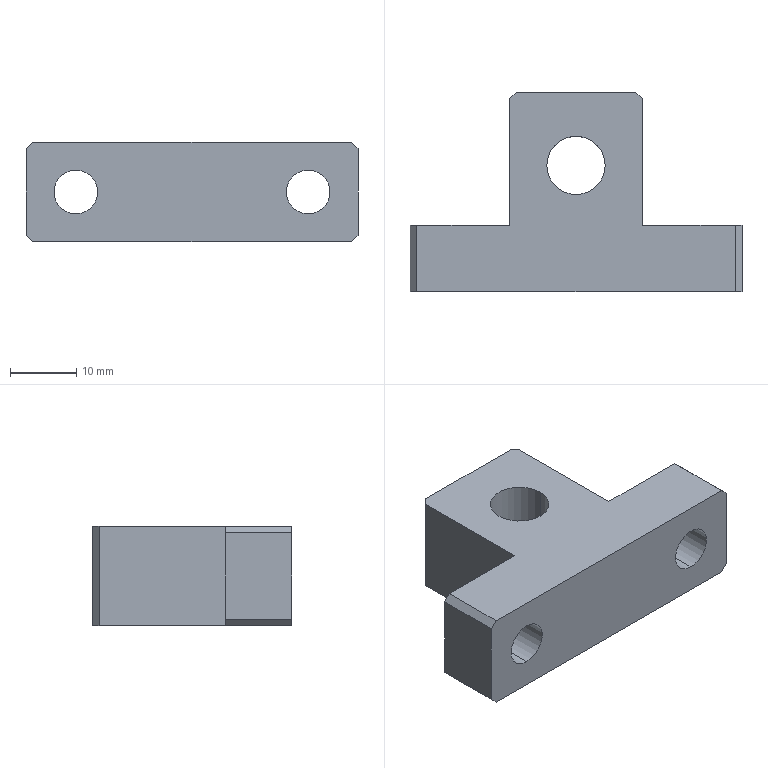Part | SolidWorks | features HoleWzd 2, Chamfer 1, Extrusion 1 | 1 solid | 22 faces | box 50 x 30 x 15 mm | volume 11868 mm3 | plane 16 | cylinder 6 | commonest cylinder face diameters 6.6 x4 8.8 x2
STEP:
#1=CARTESIAN_POINT('',(-2.322,10.722,0.));
#2=VERTEX_POINT('',#1);
#3=CARTESIAN_POINT('',(6.478,10.722,0.));
#4=VERTEX_POINT('',#3);
#5=CARTESIAN_POINT('',(2.078,10.722,0.));
#6=DIRECTION('',(0.,0.,1.));
#7=DIRECTION('',(1.,0.,0.));
#8=AXIS2_PLACEMENT_3D('',#5,#6,#7);
#9=CIRCLE('',#8,4.4);
#10=EDGE_CURVE('',#2,#4,#9,.T.);
#11=ORIENTED_EDGE('',*,*,#10,.F.);
#12=CARTESIAN_POINT('',(-2.322,10.722,15.));
#13=VERTEX_POINT('',#12);
#14=CARTESIAN_POINT('',(-2.322,10.722,15.));
#15=DIRECTION('',(0.,0.,1.));
#16=VECTOR('',#15,1000.);
#17=LINE('',#14,#16);
#18=EDGE_CURVE('',#2,#13,#17,.T.);
#19=ORIENTED_EDGE('',*,*,#18,.T.);
#20=CARTESIAN_POINT('',(6.478,10.722,15.));
#21=VERTEX_POINT('',#20);
#22=CARTESIAN_POINT('',(2.078,10.722,15.));
#23=DIRECTION('',(0.,0.,1.));
#24=DIRECTION('',(1.,0.,0.));
#25=AXIS2_PLACEMENT_3D('',#22,#23,#24);
#26=CIRCLE('',#25,4.4);
#27=EDGE_CURVE('',#13,#21,#26,.T.);
#28=ORIENTED_EDGE('',*,*,#27,.T.);
#29=CARTESIAN_POINT('',(6.478,10.722,15.));
#30=DIRECTION('',(0.,0.,1.));
#31=VECTOR('',#30,1000.);
#32=LINE('',#29,#31);
#33=EDGE_CURVE('',#4,#21,#32,.T.);
#34=ORIENTED_EDGE('',*,*,#33,.F.);
#35=EDGE_LOOP('',(#11,#19,#28,#34));
#36=FACE_OUTER_BOUND('',#35,.T.);
#37=CARTESIAN_POINT('',(2.078,10.722,15.));
#38=DIRECTION('',(0.,0.,1.));
#39=DIRECTION('',(1.,0.,0.));
#40=AXIS2_PLACEMENT_3D('',#37,#38,#39);
#41=CYLINDRICAL_SURFACE('',#40,4.4);
#42=ADVANCED_FACE('',(#36),#41,.F.);
#43=CARTESIAN_POINT('',(-15.422,-8.278,4.2));
#44=VERTEX_POINT('',#43);
#45=CARTESIAN_POINT('',(-15.422,-8.278,10.8));
#46=VERTEX_POINT('',#45);
#47=CARTESIAN_POINT('',(-15.422,-8.278,7.5));
#48=DIRECTION('',(0.,1.,0.));
#49=DIRECTION('',(0.,0.,1.));
#50=AXIS2_PLACEMENT_3D('',#47,#48,#49);
#51=CIRCLE('',#50,3.3);
#52=EDGE_CURVE('',#44,#46,#51,.T.);
#53=ORIENTED_EDGE('',*,*,#52,.F.);
#54=CARTESIAN_POINT('',(-15.422,1.722,4.2));
#55=VERTEX_POINT('',#54);
#56=CARTESIAN_POINT('',(-15.422,1.722,4.2));
#57=DIRECTION('',(0.,1.,0.));
#58=VECTOR('',#57,1000.);
#59=LINE('',#56,#58);
#60=EDGE_CURVE('',#44,#55,#59,.T.);
#61=ORIENTED_EDGE('',*,*,#60,.T.);
#62=CARTESIAN_POINT('',(-15.422,1.722,10.8));
#63=VERTEX_POINT('',#62);
#64=CARTESIAN_POINT('',(-15.422,1.722,7.5));
#65=DIRECTION('',(0.,1.,0.));
#66=DIRECTION('',(0.,0.,1.));
#67=AXIS2_PLACEMENT_3D('',#64,#65,#66);
#68=CIRCLE('',#67,3.3);
#69=EDGE_CURVE('',#55,#63,#68,.T.);
#70=ORIENTED_EDGE('',*,*,#69,.T.);
#71=CARTESIAN_POINT('',(-15.422,1.722,10.8));
#72=DIRECTION('',(0.,1.,0.));
#73=VECTOR('',#72,1000.);
#74=LINE('',#71,#73);
#75=EDGE_CURVE('',#46,#63,#74,.T.);
#76=ORIENTED_EDGE('',*,*,#75,.F.);
#77=EDGE_LOOP('',(#53,#61,#70,#76));
#78=FACE_OUTER_BOUND('',#77,.T.);
#79=CARTESIAN_POINT('',(-15.422,1.722,7.5));
#80=DIRECTION('',(0.,1.,0.));
#81=DIRECTION('',(0.,0.,1.));
#82=AXIS2_PLACEMENT_3D('',#79,#80,#81);
#83=CYLINDRICAL_SURFACE('',#82,3.3);
#84=ADVANCED_FACE('',(#78),#83,.F.);
#85=CARTESIAN_POINT('',(19.578,-8.278,4.2));
#86=VERTEX_POINT('',#85);
#87=CARTESIAN_POINT('',(19.578,-8.278,10.8));
#88=VERTEX_POINT('',#87);
#89=CARTESIAN_POINT('',(19.578,-8.278,7.5));
#90=DIRECTION('',(0.,1.,0.));
#91=DIRECTION('',(0.,0.,1.));
#92=AXIS2_PLACEMENT_3D('',#89,#90,#91);
#93=CIRCLE('',#92,3.3);
#94=EDGE_CURVE('',#86,#88,#93,.T.);
#95=ORIENTED_EDGE('',*,*,#94,.F.);
#96=CARTESIAN_POINT('',(19.578,1.722,4.2));
#97=VERTEX_POINT('',#96);
#98=CARTESIAN_POINT('',(19.578,1.722,4.2));
#99=DIRECTION('',(0.,1.,0.));
#100=VECTOR('',#99,1000.);
#101=LINE('',#98,#100);
#102=EDGE_CURVE('',#86,#97,#101,.T.);
#103=ORIENTED_EDGE('',*,*,#102,.T.);
#104=CARTESIAN_POINT('',(19.578,1.722,10.8));
#105=VERTEX_POINT('',#104);
#106=CARTESIAN_POINT('',(19.578,1.722,7.5));
#107=DIRECTION('',(0.,1.,0.));
#108=DIRECTION('',(0.,0.,1.));
#109=AXIS2_PLACEMENT_3D('',#106,#107,#108);
#110=CIRCLE('',#109,3.3);
#111=EDGE_CURVE('',#97,#105,#110,.T.);
#112=ORIENTED_EDGE('',*,*,#111,.T.);
#113=CARTESIAN_POINT('',(19.578,1.722,10.8));
#114=DIRECTION('',(0.,1.,0.));
#115=VECTOR('',#114,1000.);
#116=LINE('',#113,#115);
#117=EDGE_CURVE('',#88,#105,#116,.T.);
#118=ORIENTED_EDGE('',*,*,#117,.F.);
#119=EDGE_LOOP('',(#95,#103,#112,#118));
#120=FACE_OUTER_BOUND('',#119,.T.);
#121=CARTESIAN_POINT('',(19.578,1.722,7.5));
#122=DIRECTION('',(0.,1.,0.));
#123=DIRECTION('',(0.,0.,1.));
#124=AXIS2_PLACEMENT_3D('',#121,#122,#123);
#125=CYLINDRICAL_SURFACE('',#124,3.3);
#126=ADVANCED_FACE('',(#120),#125,.F.);
#127=CARTESIAN_POINT('',(11.078,21.722,15.));
#128=VERTEX_POINT('',#127);
#129=CARTESIAN_POINT('',(-6.922,21.722,15.));
#130=VERTEX_POINT('',#129);
#131=CARTESIAN_POINT('',(12.078,21.722,15.));
#132=DIRECTION('',(-1.,0.,0.));
#133=VECTOR('',#132,1000.);
#134=LINE('',#131,#133);
#135=EDGE_CURVE('',#128,#130,#134,.T.);
#136=ORIENTED_EDGE('',*,*,#135,.F.);
#137=CARTESIAN_POINT('',(11.078,21.722,0.));
#138=VERTEX_POINT('',#137);
#139=CARTESIAN_POINT('',(11.078,21.722,15.));
#140=DIRECTION('',(0.,0.,-1.));
#141=VECTOR('',#140,1000.);
#142=LINE('',#139,#141);
#143=EDGE_CURVE('',#128,#138,#142,.T.);
#144=ORIENTED_EDGE('',*,*,#143,.T.);
#145=CARTESIAN_POINT('',(-6.922,21.722,0.));
#146=VERTEX_POINT('',#145);
#147=CARTESIAN_POINT('',(12.078,21.722,0.));
#148=DIRECTION('',(-1.,0.,0.));
#149=VECTOR('',#148,1000.);
#150=LINE('',#147,#149);
#151=EDGE_CURVE('',#138,#146,#150,.T.);
#152=ORIENTED_EDGE('',*,*,#151,.T.);
#153=CARTESIAN_POINT('',(-6.922,21.722,15.));
#154=DIRECTION('',(0.,0.,1.));
#155=VECTOR('',#154,1000.);
#156=LINE('',#153,#155);
#157=EDGE_CURVE('',#146,#130,#156,.T.);
#158=ORIENTED_EDGE('',*,*,#157,.T.);
#159=EDGE_LOOP('',(#136,#144,#152,#158));
#160=FACE_OUTER_BOUND('',#159,.T.);
#161=CARTESIAN_POINT('',(12.078,21.722,15.));
#162=DIRECTION('',(0.,-1.,0.));
#163=DIRECTION('',(1.,0.,0.));
#164=AXIS2_PLACEMENT_3D('',#161,#162,#163);
#165=PLANE('',#164);
#166=ADVANCED_FACE('',(#160),#165,.F.);
#167=CARTESIAN_POINT('',(-7.922,20.722,15.));
#168=VERTEX_POINT('',#167);
#169=CARTESIAN_POINT('',(-7.922,1.722,15.));
#170=VERTEX_POINT('',#169);
#171=CARTESIAN_POINT('',(-7.922,21.722,15.));
#172=DIRECTION('',(0.,-1.,0.));
#173=VECTOR('',#172,1000.);
#174=LINE('',#171,#173);
#175=EDGE_CURVE('',#168,#170,#174,.T.);
#176=ORIENTED_EDGE('',*,*,#175,.F.);
#177=CARTESIAN_POINT('',(-7.922,20.722,0.));
#178=VERTEX_POINT('',#177);
#179=CARTESIAN_POINT('',(-7.922,20.722,15.));
#180=DIRECTION('',(0.,0.,-1.));
#181=VECTOR('',#180,1000.);
#182=LINE('',#179,#181);
#183=EDGE_CURVE('',#168,#178,#182,.T.);
#184=ORIENTED_EDGE('',*,*,#183,.T.);
#185=CARTESIAN_POINT('',(-7.922,1.722,0.));
#186=VERTEX_POINT('',#185);
#187=CARTESIAN_POINT('',(-7.922,21.722,0.));
#188=DIRECTION('',(0.,-1.,0.));
#189=VECTOR('',#188,1000.);
#190=LINE('',#187,#189);
#191=EDGE_CURVE('',#178,#186,#190,.T.);
#192=ORIENTED_EDGE('',*,*,#191,.T.);
#193=CARTESIAN_POINT('',(-7.922,1.722,15.));
#194=DIRECTION('',(0.,0.,-1.));
#195=VECTOR('',#194,1000.);
#196=LINE('',#193,#195);
#197=EDGE_CURVE('',#170,#186,#196,.T.);
#198=ORIENTED_EDGE('',*,*,#197,.F.);
#199=EDGE_LOOP('',(#176,#184,#192,#198));
#200=FACE_OUTER_BOUND('',#199,.T.);
#201=CARTESIAN_POINT('',(-7.922,21.722,15.));
#202=DIRECTION('',(1.,0.,0.));
#203=DIRECTION('',(0.,1.,0.));
#204=AXIS2_PLACEMENT_3D('',#201,#202,#203);
#205=PLANE('',#204);
#206=ADVANCED_FACE('',(#200),#205,.F.);
#207=CARTESIAN_POINT('',(-15.422,1.722,7.5));
#208=DIRECTION('',(0.,1.,0.));
#209=DIRECTION('',(0.,0.,1.));
#210=AXIS2_PLACEMENT_3D('',#207,#208,#209);
#211=CIRCLE('',#210,3.3);
#212=EDGE_CURVE('',#63,#55,#211,.T.);
#213=ORIENTED_EDGE('',*,*,#212,.F.);
#214=ORIENTED_EDGE('',*,*,#69,.F.);
#215=EDGE_LOOP('',(#213,#214));
#216=FACE_BOUND('',#215,.T.);
#217=CARTESIAN_POINT('',(-22.922,1.722,14.));
#218=VERTEX_POINT('',#217);
#219=CARTESIAN_POINT('',(-22.922,1.722,1.));
#220=VERTEX_POINT('',#219);
#221=CARTESIAN_POINT('',(-22.922,1.722,15.));
#222=DIRECTION('',(0.,0.,-1.));
#223=VECTOR('',#222,1000.);
#224=LINE('',#221,#223);
#225=EDGE_CURVE('',#218,#220,#224,.T.);
#226=ORIENTED_EDGE('',*,*,#225,.F.);
#227=CARTESIAN_POINT('',(-21.922,1.722,15.));
#228=VERTEX_POINT('',#227);
#229=CARTESIAN_POINT('',(-21.922,1.722,15.));
#230=DIRECTION('',(0.7071,0.,0.7071));
#231=VECTOR('',#230,1000.);
#232=LINE('',#229,#231);
#233=EDGE_CURVE('',#218,#228,#232,.T.);
#234=ORIENTED_EDGE('',*,*,#233,.T.);
#235=CARTESIAN_POINT('',(-7.922,1.722,15.));
#236=DIRECTION('',(-1.,0.,0.));
#237=VECTOR('',#236,1000.);
#238=LINE('',#235,#237);
#239=EDGE_CURVE('',#170,#228,#238,.T.);
#240=ORIENTED_EDGE('',*,*,#239,.F.);
#241=ORIENTED_EDGE('',*,*,#197,.T.);
#242=CARTESIAN_POINT('',(-21.922,1.722,0.));
#243=VERTEX_POINT('',#242);
#244=CARTESIAN_POINT('',(-7.922,1.722,0.));
#245=DIRECTION('',(-1.,0.,0.));
#246=VECTOR('',#245,1000.);
#247=LINE('',#244,#246);
#248=EDGE_CURVE('',#186,#243,#247,.T.);
#249=ORIENTED_EDGE('',*,*,#248,.T.);
#250=CARTESIAN_POINT('',(-22.922,1.722,1.));
#251=DIRECTION('',(-0.7071,0.,0.7071));
#252=VECTOR('',#251,1000.);
#253=LINE('',#250,#252);
#254=EDGE_CURVE('',#243,#220,#253,.T.);
#255=ORIENTED_EDGE('',*,*,#254,.T.);
#256=EDGE_LOOP('',(#226,#234,#240,#241,#249,#255));
#257=FACE_OUTER_BOUND('',#256,.T.);
#258=CARTESIAN_POINT('',(-7.922,1.722,15.));
#259=DIRECTION('',(0.,-1.,0.));
#260=DIRECTION('',(1.,0.,0.));
#261=AXIS2_PLACEMENT_3D('',#258,#259,#260);
#262=PLANE('',#261);
#263=ADVANCED_FACE('',(#216,#257),#262,.F.);
#264=CARTESIAN_POINT('',(-22.922,-8.278,14.));
#265=VERTEX_POINT('',#264);
#266=CARTESIAN_POINT('',(-22.922,-8.278,1.));
#267=VERTEX_POINT('',#266);
#268=CARTESIAN_POINT('',(-22.922,-8.278,15.));
#269=DIRECTION('',(0.,0.,-1.));
#270=VECTOR('',#269,1000.);
#271=LINE('',#268,#270);
#272=EDGE_CURVE('',#265,#267,#271,.T.);
#273=ORIENTED_EDGE('',*,*,#272,.F.);
#274=CARTESIAN_POINT('',(-22.922,1.722,14.));
#275=DIRECTION('',(0.,1.,0.));
#276=VECTOR('',#275,1000.);
#277=LINE('',#274,#276);
#278=EDGE_CURVE('',#265,#218,#277,.T.);
#279=ORIENTED_EDGE('',*,*,#278,.T.);
#280=ORIENTED_EDGE('',*,*,#225,.T.);
#281=CARTESIAN_POINT('',(-22.922,1.722,1.));
#282=DIRECTION('',(0.,-1.,0.));
#283=VECTOR('',#282,1000.);
#284=LINE('',#281,#283);
#285=EDGE_CURVE('',#220,#267,#284,.T.);
#286=ORIENTED_EDGE('',*,*,#285,.T.);
#287=EDGE_LOOP('',(#273,#279,#280,#286));
#288=FACE_OUTER_BOUND('',#287,.T.);
#289=CARTESIAN_POINT('',(-22.922,1.722,15.));
#290=DIRECTION('',(1.,0.,0.));
#291=DIRECTION('',(0.,0.,-1.));
#292=AXIS2_PLACEMENT_3D('',#289,#290,#291);
#293=PLANE('',#292);
#294=ADVANCED_FACE('',(#288),#293,.F.);
#295=CARTESIAN_POINT('',(-15.422,-8.278,7.5));
#296=DIRECTION('',(0.,1.,0.));
#297=DIRECTION('',(0.,0.,1.));
#298=AXIS2_PLACEMENT_3D('',#295,#296,#297);
#299=CIRCLE('',#298,3.3);
#300=EDGE_CURVE('',#46,#44,#299,.T.);
#301=ORIENTED_EDGE('',*,*,#300,.T.);
#302=ORIENTED_EDGE('',*,*,#52,.T.);
#303=EDGE_LOOP('',(#301,#302));
#304=FACE_BOUND('',#303,.T.);
#305=CARTESIAN_POINT('',(19.578,-8.278,7.5));
#306=DIRECTION('',(0.,1.,0.));
#307=DIRECTION('',(0.,0.,1.));
#308=AXIS2_PLACEMENT_3D('',#305,#306,#307);
#309=CIRCLE('',#308,3.3);
#310=EDGE_CURVE('',#88,#86,#309,.T.);
#311=ORIENTED_EDGE('',*,*,#310,.T.);
#312=ORIENTED_EDGE('',*,*,#94,.T.);
#313=EDGE_LOOP('',(#311,#312));
#314=FACE_BOUND('',#313,.T.);
#315=CARTESIAN_POINT('',(27.078,-8.278,14.));
#316=VERTEX_POINT('',#315);
#317=CARTESIAN_POINT('',(27.078,-8.278,1.));
#318=VERTEX_POINT('',#317);
#319=CARTESIAN_POINT('',(27.078,-8.278,15.));
#320=DIRECTION('',(0.,0.,-1.));
#321=VECTOR('',#320,1000.);
#322=LINE('',#319,#321);
#323=EDGE_CURVE('',#316,#318,#322,.T.);
#324=ORIENTED_EDGE('',*,*,#323,.F.);
#325=CARTESIAN_POINT('',(26.078,-8.278,15.));
#326=VERTEX_POINT('',#325);
#327=CARTESIAN_POINT('',(26.078,-8.278,15.));
#328=DIRECTION('',(-0.7071,0.,0.7071));
#329=VECTOR('',#328,1000.);
#330=LINE('',#327,#329);
#331=EDGE_CURVE('',#316,#326,#330,.T.);
#332=ORIENTED_EDGE('',*,*,#331,.T.);
#333=CARTESIAN_POINT('',(-21.922,-8.278,15.));
#334=VERTEX_POINT('',#333);
#335=CARTESIAN_POINT('',(-22.922,-8.278,15.));
#336=DIRECTION('',(1.,0.,0.));
#337=VECTOR('',#336,1000.);
#338=LINE('',#335,#337);
#339=EDGE_CURVE('',#334,#326,#338,.T.);
#340=ORIENTED_EDGE('',*,*,#339,.F.);
#341=CARTESIAN_POINT('',(-21.922,-8.278,15.));
#342=DIRECTION('',(-0.7071,0.,-0.7071));
#343=VECTOR('',#342,1000.);
#344=LINE('',#341,#343);
#345=EDGE_CURVE('',#334,#265,#344,.T.);
#346=ORIENTED_EDGE('',*,*,#345,.T.);
#347=ORIENTED_EDGE('',*,*,#272,.T.);
#348=CARTESIAN_POINT('',(-21.922,-8.278,0.));
#349=VERTEX_POINT('',#348);
#350=CARTESIAN_POINT('',(-22.922,-8.278,1.));
#351=DIRECTION('',(0.7071,0.,-0.7071));
#352=VECTOR('',#351,1000.);
#353=LINE('',#350,#352);
#354=EDGE_CURVE('',#267,#349,#353,.T.);
#355=ORIENTED_EDGE('',*,*,#354,.T.);
#356=CARTESIAN_POINT('',(26.078,-8.278,0.));
#357=VERTEX_POINT('',#356);
#358=CARTESIAN_POINT('',(-22.922,-8.278,0.));
#359=DIRECTION('',(1.,0.,0.));
#360=VECTOR('',#359,1000.);
#361=LINE('',#358,#360);
#362=EDGE_CURVE('',#349,#357,#361,.T.);
#363=ORIENTED_EDGE('',*,*,#362,.T.);
#364=CARTESIAN_POINT('',(27.078,-8.278,1.));
#365=DIRECTION('',(0.7071,0.,0.7071));
#366=VECTOR('',#365,1000.);
#367=LINE('',#364,#366);
#368=EDGE_CURVE('',#357,#318,#367,.T.);
#369=ORIENTED_EDGE('',*,*,#368,.T.);
#370=EDGE_LOOP('',(#324,#332,#340,#346,#347,#355,#363,#369));
#371=FACE_OUTER_BOUND('',#370,.T.);
#372=CARTESIAN_POINT('',(-22.922,-8.278,15.));
#373=DIRECTION('',(0.,1.,0.));
#374=DIRECTION('',(0.,0.,1.));
#375=AXIS2_PLACEMENT_3D('',#372,#373,#374);
#376=PLANE('',#375);
#377=ADVANCED_FACE('',(#304,#314,#371),#376,.F.);
#378=CARTESIAN_POINT('',(27.078,1.722,14.));
#379=VERTEX_POINT('',#378);
#380=CARTESIAN_POINT('',(27.078,1.722,1.));
#381=VERTEX_POINT('',#380);
#382=CARTESIAN_POINT('',(27.078,1.722,15.));
#383=DIRECTION('',(0.,0.,-1.));
#384=VECTOR('',#383,1000.);
#385=LINE('',#382,#384);
#386=EDGE_CURVE('',#379,#381,#385,.T.);
#387=ORIENTED_EDGE('',*,*,#386,.F.);
#388=CARTESIAN_POINT('',(27.078,-8.278,14.));
#389=DIRECTION('',(0.,-1.,0.));
#390=VECTOR('',#389,1000.);
#391=LINE('',#388,#390);
#392=EDGE_CURVE('',#379,#316,#391,.T.);
#393=ORIENTED_EDGE('',*,*,#392,.T.);
#394=ORIENTED_EDGE('',*,*,#323,.T.);
#395=CARTESIAN_POINT('',(27.078,-8.278,1.));
#396=DIRECTION('',(0.,1.,0.));
#397=VECTOR('',#396,1000.);
#398=LINE('',#395,#397);
#399=EDGE_CURVE('',#318,#381,#398,.T.);
#400=ORIENTED_EDGE('',*,*,#399,.T.);
#401=EDGE_LOOP('',(#387,#393,#394,#400));
#402=FACE_OUTER_BOUND('',#401,.T.);
#403=CARTESIAN_POINT('',(27.078,-8.278,15.));
#404=DIRECTION('',(-1.,0.,0.));
#405=DIRECTION('',(0.,0.,1.));
#406=AXIS2_PLACEMENT_3D('',#403,#404,#405);
#407=PLANE('',#406);
#408=ADVANCED_FACE('',(#402),#407,.F.);
#409=CARTESIAN_POINT('',(19.578,1.722,7.5));
#410=DIRECTION('',(0.,1.,0.));
#411=DIRECTION('',(0.,0.,1.));
#412=AXIS2_PLACEMENT_3D('',#409,#410,#411);
#413=CIRCLE('',#412,3.3);
#414=EDGE_CURVE('',#105,#97,#413,.T.);
#415=ORIENTED_EDGE('',*,*,#414,.F.);
#416=ORIENTED_EDGE('',*,*,#111,.F.);
#417=EDGE_LOOP('',(#415,#416));
#418=FACE_BOUND('',#417,.T.);
#419=CARTESIAN_POINT('',(26.078,1.722,15.));
#420=VERTEX_POINT('',#419);
#421=CARTESIAN_POINT('',(12.078,1.722,15.));
#422=VERTEX_POINT('',#421);
#423=CARTESIAN_POINT('',(27.078,1.722,15.));
#424=DIRECTION('',(-1.,0.,0.));
#425=VECTOR('',#424,1000.);
#426=LINE('',#423,#425);
#427=EDGE_CURVE('',#420,#422,#426,.T.);
#428=ORIENTED_EDGE('',*,*,#427,.F.);
#429=CARTESIAN_POINT('',(26.078,1.722,15.));
#430=DIRECTION('',(0.7071,0.,-0.7071));
#431=VECTOR('',#430,1000.);
#432=LINE('',#429,#431);
#433=EDGE_CURVE('',#420,#379,#432,.T.);
#434=ORIENTED_EDGE('',*,*,#433,.T.);
#435=ORIENTED_EDGE('',*,*,#386,.T.);
#436=CARTESIAN_POINT('',(26.078,1.722,0.));
#437=VERTEX_POINT('',#436);
#438=CARTESIAN_POINT('',(27.078,1.722,1.));
#439=DIRECTION('',(-0.7071,0.,-0.7071));
#440=VECTOR('',#439,1000.);
#441=LINE('',#438,#440);
#442=EDGE_CURVE('',#381,#437,#441,.T.);
#443=ORIENTED_EDGE('',*,*,#442,.T.);
#444=CARTESIAN_POINT('',(12.078,1.722,0.));
#445=VERTEX_POINT('',#444);
#446=CARTESIAN_POINT('',(27.078,1.722,0.));
#447=DIRECTION('',(-1.,0.,0.));
#448=VECTOR('',#447,1000.);
#449=LINE('',#446,#448);
#450=EDGE_CURVE('',#437,#445,#449,.T.);
#451=ORIENTED_EDGE('',*,*,#450,.T.);
#452=CARTESIAN_POINT('',(12.078,1.722,15.));
#453=DIRECTION('',(0.,0.,-1.));
#454=VECTOR('',#453,1000.);
#455=LINE('',#452,#454);
#456=EDGE_CURVE('',#422,#445,#455,.T.);
#457=ORIENTED_EDGE('',*,*,#456,.F.);
#458=EDGE_LOOP('',(#428,#434,#435,#443,#451,#457));
#459=FACE_OUTER_BOUND('',#458,.T.);
#460=CARTESIAN_POINT('',(27.078,1.722,15.));
#461=DIRECTION('',(0.,-1.,0.));
#462=DIRECTION('',(1.,0.,0.));
#463=AXIS2_PLACEMENT_3D('',#460,#461,#462);
#464=PLANE('',#463);
#465=ADVANCED_FACE('',(#418,#459),#464,.F.);
#466=CARTESIAN_POINT('',(12.078,20.722,0.));
#467=VERTEX_POINT('',#466);
#468=CARTESIAN_POINT('',(12.078,1.722,0.));
#469=DIRECTION('',(0.,1.,0.));
#470=VECTOR('',#469,1000.);
#471=LINE('',#468,#470);
#472=EDGE_CURVE('',#445,#467,#471,.T.);
#473=ORIENTED_EDGE('',*,*,#472,.T.);
#474=CARTESIAN_POINT('',(12.078,20.722,15.));
#475=VERTEX_POINT('',#474);
#476=CARTESIAN_POINT('',(12.078,20.722,15.));
#477=DIRECTION('',(0.,0.,1.));
#478=VECTOR('',#477,1000.);
#479=LINE('',#476,#478);
#480=EDGE_CURVE('',#467,#475,#479,.T.);
#481=ORIENTED_EDGE('',*,*,#480,.T.);
#482=CARTESIAN_POINT('',(12.078,1.722,15.));
#483=DIRECTION('',(0.,1.,0.));
#484=VECTOR('',#483,1000.);
#485=LINE('',#482,#484);
#486=EDGE_CURVE('',#422,#475,#485,.T.);
#487=ORIENTED_EDGE('',*,*,#486,.F.);
#488=ORIENTED_EDGE('',*,*,#456,.T.);
#489=EDGE_LOOP('',(#473,#481,#487,#488));
#490=FACE_OUTER_BOUND('',#489,.T.);
#491=CARTESIAN_POINT('',(12.078,1.722,15.));
#492=DIRECTION('',(-1.,0.,0.));
#493=DIRECTION('',(0.,0.,1.));
#494=AXIS2_PLACEMENT_3D('',#491,#492,#493);
#495=PLANE('',#494);
#496=ADVANCED_FACE('',(#490),#495,.F.);
#497=CARTESIAN_POINT('',(2.078,10.722,15.));
#498=DIRECTION('',(0.,0.,1.));
#499=DIRECTION('',(1.,0.,0.));
#500=AXIS2_PLACEMENT_3D('',#497,#498,#499);
#501=CIRCLE('',#500,4.4);
#502=EDGE_CURVE('',#21,#13,#501,.T.);
#503=ORIENTED_EDGE('',*,*,#502,.F.);
#504=ORIENTED_EDGE('',*,*,#27,.F.);
#505=EDGE_LOOP('',(#503,#504));
#506=FACE_BOUND('',#505,.T.);
#507=ORIENTED_EDGE('',*,*,#339,.T.);
#508=CARTESIAN_POINT('',(26.078,1.722,15.));
#509=DIRECTION('',(0.,1.,0.));
#510=VECTOR('',#509,1000.);
#511=LINE('',#508,#510);
#512=EDGE_CURVE('',#326,#420,#511,.T.);
#513=ORIENTED_EDGE('',*,*,#512,.T.);
#514=ORIENTED_EDGE('',*,*,#427,.T.);
#515=ORIENTED_EDGE('',*,*,#486,.T.);
#516=CARTESIAN_POINT('',(16.4,16.4,15.));
#517=DIRECTION('',(-0.7071,0.7071,0.));
#518=VECTOR('',#517,1000.);
#519=LINE('',#516,#518);
#520=EDGE_CURVE('',#475,#128,#519,.T.);
#521=ORIENTED_EDGE('',*,*,#520,.T.);
#522=ORIENTED_EDGE('',*,*,#135,.T.);
#523=CARTESIAN_POINT('',(-14.322,14.322,15.));
#524=DIRECTION('',(-0.7071,-0.7071,0.));
#525=VECTOR('',#524,1000.);
#526=LINE('',#523,#525);
#527=EDGE_CURVE('',#130,#168,#526,.T.);
#528=ORIENTED_EDGE('',*,*,#527,.T.);
#529=ORIENTED_EDGE('',*,*,#175,.T.);
#530=ORIENTED_EDGE('',*,*,#239,.T.);
#531=CARTESIAN_POINT('',(-21.922,-8.278,15.));
#532=DIRECTION('',(0.,-1.,0.));
#533=VECTOR('',#532,1000.);
#534=LINE('',#531,#533);
#535=EDGE_CURVE('',#228,#334,#534,.T.);
#536=ORIENTED_EDGE('',*,*,#535,.T.);
#537=EDGE_LOOP('',(#507,#513,#514,#515,#521,#522,#528,#529,#530,#536));
#538=FACE_OUTER_BOUND('',#537,.T.);
#539=CARTESIAN_POINT('',(0.,0.,15.));
#540=DIRECTION('',(0.,0.,1.));
#541=DIRECTION('',(1.,0.,0.));
#542=AXIS2_PLACEMENT_3D('',#539,#540,#541);
#543=PLANE('',#542);
#544=ADVANCED_FACE('',(#506,#538),#543,.T.);
#545=CARTESIAN_POINT('',(2.078,10.722,0.));
#546=DIRECTION('',(0.,0.,1.));
#547=DIRECTION('',(1.,0.,0.));
#548=AXIS2_PLACEMENT_3D('',#545,#546,#547);
#549=CIRCLE('',#548,4.4);
#550=EDGE_CURVE('',#4,#2,#549,.T.);
#551=ORIENTED_EDGE('',*,*,#550,.T.);
#552=ORIENTED_EDGE('',*,*,#10,.T.);
#553=EDGE_LOOP('',(#551,#552));
#554=FACE_BOUND('',#553,.T.);
#555=ORIENTED_EDGE('',*,*,#450,.F.);
#556=CARTESIAN_POINT('',(26.078,0.,0.));
#557=DIRECTION('',(0.,-1.,0.));
#558=VECTOR('',#557,1000.);
#559=LINE('',#556,#558);
#560=EDGE_CURVE('',#437,#357,#559,.T.);
#561=ORIENTED_EDGE('',*,*,#560,.T.);
#562=ORIENTED_EDGE('',*,*,#362,.F.);
#563=CARTESIAN_POINT('',(-21.922,0.,0.));
#564=DIRECTION('',(0.,1.,0.));
#565=VECTOR('',#564,1000.);
#566=LINE('',#563,#565);
#567=EDGE_CURVE('',#349,#243,#566,.T.);
#568=ORIENTED_EDGE('',*,*,#567,.T.);
#569=ORIENTED_EDGE('',*,*,#248,.F.);
#570=ORIENTED_EDGE('',*,*,#191,.F.);
#571=CARTESIAN_POINT('',(-7.922,20.722,0.));
#572=DIRECTION('',(0.7071,0.7071,0.));
#573=VECTOR('',#572,1000.);
#574=LINE('',#571,#573);
#575=EDGE_CURVE('',#178,#146,#574,.T.);
#576=ORIENTED_EDGE('',*,*,#575,.T.);
#577=ORIENTED_EDGE('',*,*,#151,.F.);
#578=CARTESIAN_POINT('',(11.078,21.722,0.));
#579=DIRECTION('',(0.7071,-0.7071,0.));
#580=VECTOR('',#579,1000.);
#581=LINE('',#578,#580);
#582=EDGE_CURVE('',#138,#467,#581,.T.);
#583=ORIENTED_EDGE('',*,*,#582,.T.);
#584=ORIENTED_EDGE('',*,*,#472,.F.);
#585=EDGE_LOOP('',(#555,#561,#562,#568,#569,#570,#576,#577,#583,#584));
#586=FACE_OUTER_BOUND('',#585,.T.);
#587=CARTESIAN_POINT('',(0.,0.,0.));
#588=DIRECTION('',(0.,0.,1.));
#589=DIRECTION('',(1.,0.,0.));
#590=AXIS2_PLACEMENT_3D('',#587,#588,#589);
#591=PLANE('',#590);
#592=ADVANCED_FACE('',(#554,#586),#591,.F.);
#593=ORIENTED_EDGE('',*,*,#331,.F.);
#594=ORIENTED_EDGE('',*,*,#392,.F.);
#595=ORIENTED_EDGE('',*,*,#433,.F.);
#596=ORIENTED_EDGE('',*,*,#512,.F.);
#597=EDGE_LOOP('',(#593,#594,#595,#596));
#598=FACE_OUTER_BOUND('',#597,.T.);
#599=CARTESIAN_POINT('',(26.078,0.,15.));
#600=DIRECTION('',(0.7071,0.,0.7071));
#601=DIRECTION('',(0.,-1.,0.));
#602=AXIS2_PLACEMENT_3D('',#599,#600,#601);
#603=PLANE('',#602);
#604=ADVANCED_FACE('',(#598),#603,.T.);
#605=ORIENTED_EDGE('',*,*,#368,.F.);
#606=ORIENTED_EDGE('',*,*,#560,.F.);
#607=ORIENTED_EDGE('',*,*,#442,.F.);
#608=ORIENTED_EDGE('',*,*,#399,.F.);
#609=EDGE_LOOP('',(#605,#606,#607,#608));
#610=FACE_OUTER_BOUND('',#609,.T.);
#611=CARTESIAN_POINT('',(27.078,-8.278,1.));
#612=DIRECTION('',(-0.7071,0.,0.7071));
#613=DIRECTION('',(0.,1.,0.));
#614=AXIS2_PLACEMENT_3D('',#611,#612,#613);
#615=PLANE('',#614);
#616=ADVANCED_FACE('',(#610),#615,.F.);
#617=ORIENTED_EDGE('',*,*,#233,.F.);
#618=ORIENTED_EDGE('',*,*,#278,.F.);
#619=ORIENTED_EDGE('',*,*,#345,.F.);
#620=ORIENTED_EDGE('',*,*,#535,.F.);
#621=EDGE_LOOP('',(#617,#618,#619,#620));
#622=FACE_OUTER_BOUND('',#621,.T.);
#623=CARTESIAN_POINT('',(-21.922,0.,15.));
#624=DIRECTION('',(-0.7071,0.,0.7071));
#625=DIRECTION('',(0.,1.,0.));
#626=AXIS2_PLACEMENT_3D('',#623,#624,#625);
#627=PLANE('',#626);
#628=ADVANCED_FACE('',(#622),#627,.T.);
#629=ORIENTED_EDGE('',*,*,#254,.F.);
#630=ORIENTED_EDGE('',*,*,#567,.F.);
#631=ORIENTED_EDGE('',*,*,#354,.F.);
#632=ORIENTED_EDGE('',*,*,#285,.F.);
#633=EDGE_LOOP('',(#629,#630,#631,#632));
#634=FACE_OUTER_BOUND('',#633,.T.);
#635=CARTESIAN_POINT('',(-22.922,1.722,1.));
#636=DIRECTION('',(0.7071,0.,0.7071));
#637=DIRECTION('',(0.,-1.,0.));
#638=AXIS2_PLACEMENT_3D('',#635,#636,#637);
#639=PLANE('',#638);
#640=ADVANCED_FACE('',(#634),#639,.F.);
#641=ORIENTED_EDGE('',*,*,#520,.F.);
#642=ORIENTED_EDGE('',*,*,#480,.F.);
#643=ORIENTED_EDGE('',*,*,#582,.F.);
#644=ORIENTED_EDGE('',*,*,#143,.F.);
#645=EDGE_LOOP('',(#641,#642,#643,#644));
#646=FACE_OUTER_BOUND('',#645,.T.);
#647=CARTESIAN_POINT('',(11.078,21.722,15.));
#648=DIRECTION('',(-0.7071,-0.7071,0.));
#649=DIRECTION('',(0.,0.,-1.));
#650=AXIS2_PLACEMENT_3D('',#647,#648,#649);
#651=PLANE('',#650);
#652=ADVANCED_FACE('',(#646),#651,.F.);
#653=ORIENTED_EDGE('',*,*,#527,.F.);
#654=ORIENTED_EDGE('',*,*,#157,.F.);
#655=ORIENTED_EDGE('',*,*,#575,.F.);
#656=ORIENTED_EDGE('',*,*,#183,.F.);
#657=EDGE_LOOP('',(#653,#654,#655,#656));
#658=FACE_OUTER_BOUND('',#657,.T.);
#659=CARTESIAN_POINT('',(-7.922,20.722,15.));
#660=DIRECTION('',(0.7071,-0.7071,0.));
#661=DIRECTION('',(0.,0.,-1.));
#662=AXIS2_PLACEMENT_3D('',#659,#660,#661);
#663=PLANE('',#662);
#664=ADVANCED_FACE('',(#658),#663,.F.);
#665=ORIENTED_EDGE('',*,*,#102,.F.);
#666=ORIENTED_EDGE('',*,*,#310,.F.);
#667=ORIENTED_EDGE('',*,*,#117,.T.);
#668=ORIENTED_EDGE('',*,*,#414,.T.);
#669=EDGE_LOOP('',(#665,#666,#667,#668));
#670=FACE_OUTER_BOUND('',#669,.T.);
#671=CARTESIAN_POINT('',(19.578,1.722,7.5));
#672=DIRECTION('',(0.,1.,0.));
#673=DIRECTION('',(0.,0.,1.));
#674=AXIS2_PLACEMENT_3D('',#671,#672,#673);
#675=CYLINDRICAL_SURFACE('',#674,3.3);
#676=ADVANCED_FACE('',(#670),#675,.F.);
#677=ORIENTED_EDGE('',*,*,#60,.F.);
#678=ORIENTED_EDGE('',*,*,#300,.F.);
#679=ORIENTED_EDGE('',*,*,#75,.T.);
#680=ORIENTED_EDGE('',*,*,#212,.T.);
#681=EDGE_LOOP('',(#677,#678,#679,#680));
#682=FACE_OUTER_BOUND('',#681,.T.);
#683=CARTESIAN_POINT('',(-15.422,1.722,7.5));
#684=DIRECTION('',(0.,1.,0.));
#685=DIRECTION('',(0.,0.,1.));
#686=AXIS2_PLACEMENT_3D('',#683,#684,#685);
#687=CYLINDRICAL_SURFACE('',#686,3.3);
#688=ADVANCED_FACE('',(#682),#687,.F.);
#689=ORIENTED_EDGE('',*,*,#18,.F.);
#690=ORIENTED_EDGE('',*,*,#550,.F.);
#691=ORIENTED_EDGE('',*,*,#33,.T.);
#692=ORIENTED_EDGE('',*,*,#502,.T.);
#693=EDGE_LOOP('',(#689,#690,#691,#692));
#694=FACE_OUTER_BOUND('',#693,.T.);
#695=CARTESIAN_POINT('',(2.078,10.722,15.));
#696=DIRECTION('',(0.,0.,1.));
#697=DIRECTION('',(1.,0.,0.));
#698=AXIS2_PLACEMENT_3D('',#695,#696,#697);
#699=CYLINDRICAL_SURFACE('',#698,4.4);
#700=ADVANCED_FACE('',(#694),#699,.F.);
#701=CLOSED_SHELL('',(#42,#84,#126,#166,#206,#263,#294,#377,#408,#465,#496,#544,#592,#604,#616,#628,#640,#652,#664,#676,#688,#700));
#702=MANIFOLD_SOLID_BREP('',#701);
#703=CARTESIAN_POINT('',(0.,0.,0.));
#704=DIRECTION('',(0.,0.,1.));
#705=DIRECTION('',(1.,0.,0.));
#706=AXIS2_PLACEMENT_3D('',#703,#704,#705);
#707=(LENGTH_UNIT()NAMED_UNIT(*)SI_UNIT(.MILLI.,.METRE.));
#708=UNCERTAINTY_MEASURE_WITH_UNIT(LENGTH_MEASURE(0.00001),#707,'','');
#709=(NAMED_UNIT(*)PLANE_ANGLE_UNIT()SI_UNIT($,.RADIAN.));
#710=(NAMED_UNIT(*)SI_UNIT($,.STERADIAN.)SOLID_ANGLE_UNIT());
#711=(GEOMETRIC_REPRESENTATION_CONTEXT(3)GLOBAL_UNCERTAINTY_ASSIGNED_CONTEXT((#708))GLOBAL_UNIT_ASSIGNED_CONTEXT((#707,#709,#710))REPRESENTATION_CONTEXT('',''));
#712=ADVANCED_BREP_SHAPE_REPRESENTATION('',(#702,#706),#711);